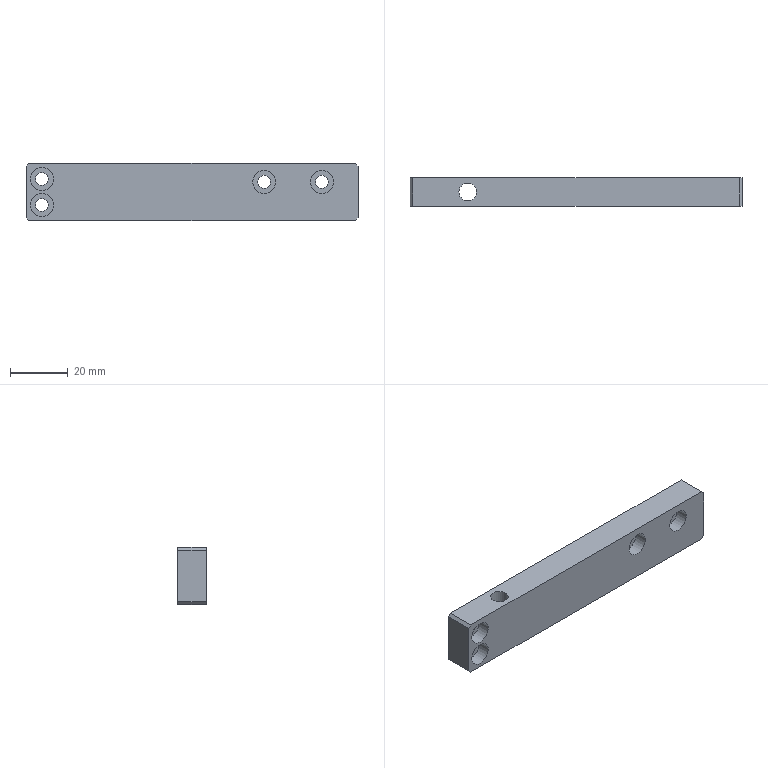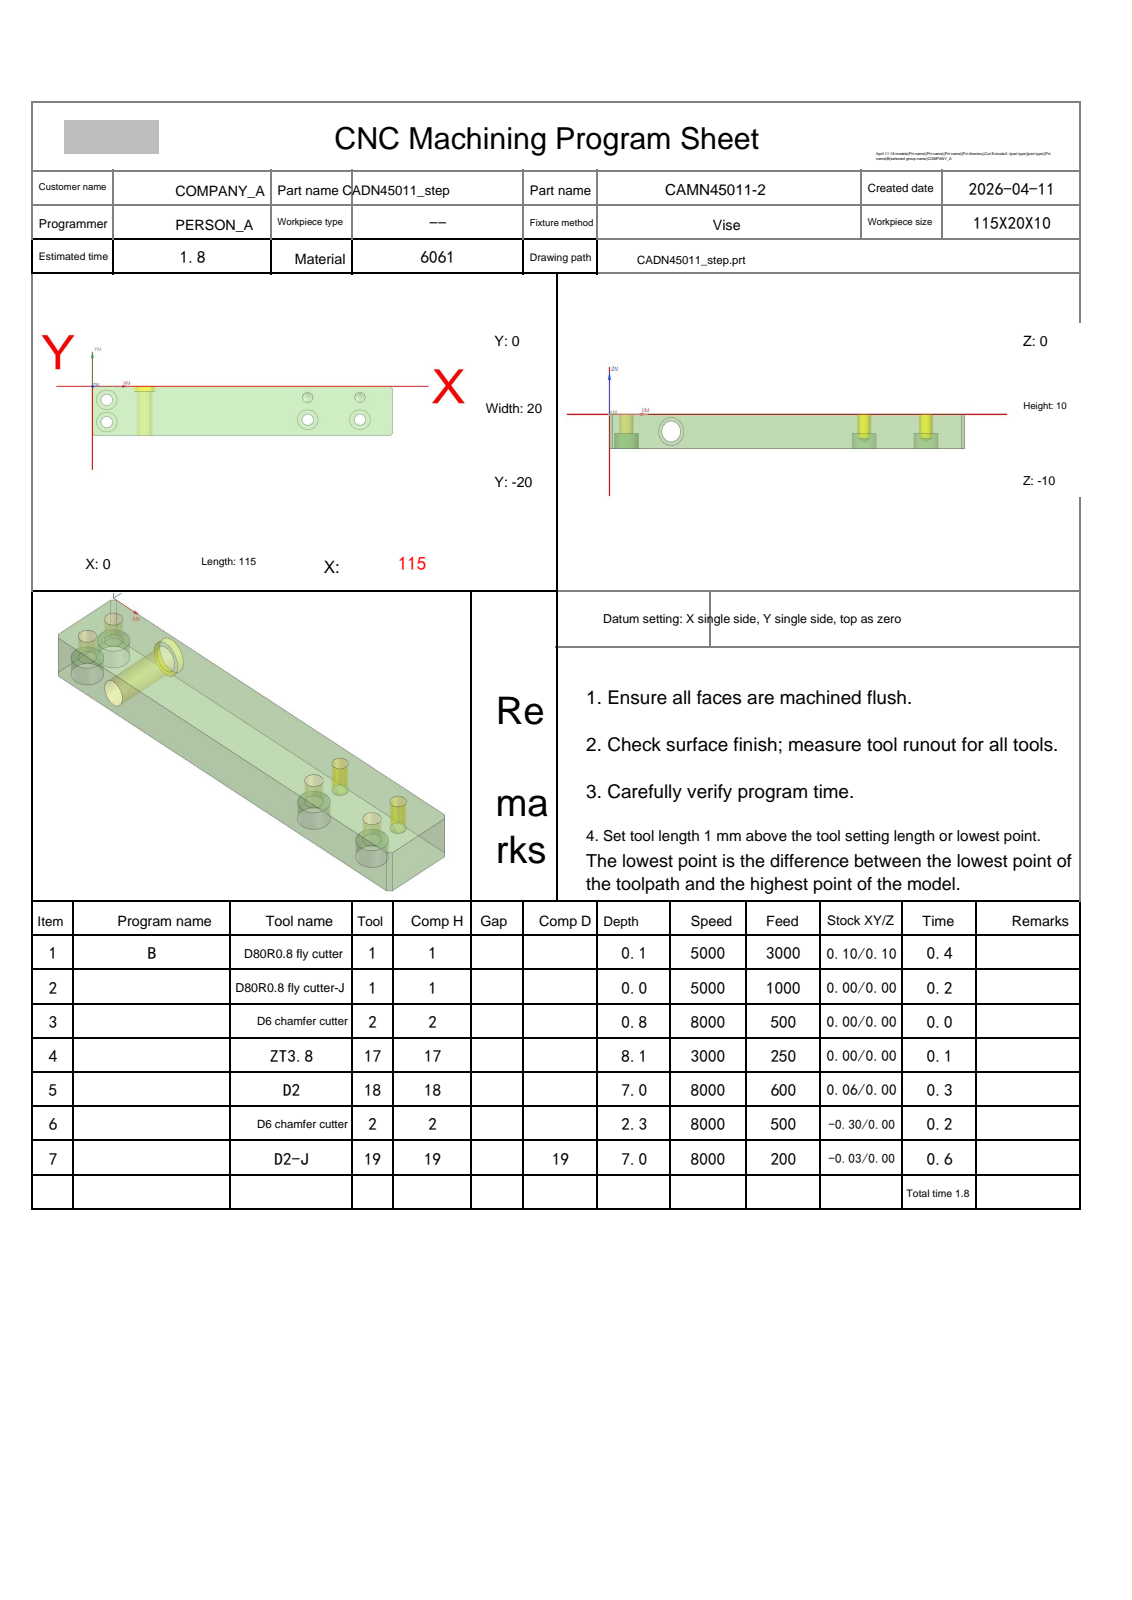NC program | NX | posted by the shop | part box 115 x 10 x 20 mm
Whole program:
%
O0001
(Machine time: 3.22 MIN)
(===Total Tool:5===)
(T1=D80R0.8 fly cutter D=80.  R=0.8  D-  H01 Z=0.    )
(T2=D6 chamfer cutter   D=6.   R=0.   D-  H02 Z=-2.3  )
(T17=ZT3.8  D=3.8  DR_a=118 D-  H17 Z=-8.1  )
(T18=D2     D=2.   R=0.   D-  H18 Z=-7.   )
(T19=D2-J   D=2.   R=0.   D19 H19 Z=-7.   )
G80 G90 G17 G49 G40
G91 G28 Z0
M01
N1 T01 M06
(D80R0.8 fly cutter  D=80. R=0.8 H=01 ce=0.10 di=0.10)
G00 G90 G54 X167.097 Y-10. M03 S5000
G43 H01 Z20.
M08
Z3.525
G01 Z1.525 F3000.
X155.097
X-40.097
X-52.097
Z3.525
G00 X167.097
Z3.05
G01 Z1.05
X155.097
X-40.097
X-52.097
Z3.05
G00 X167.097
Z2.575
G01 Z.575
X155.097
X-40.097
X-52.097
Z2.575
G00 X167.097
Z2.1
G01 Z.1
X155.097
X-40.097
X-52.097
Z2.1
G00 Z20.
G91 G28 Z0.0
M05
M09
G91 G28 Z0.0
M01
N2 T01 M06
(D80R0.8 fly cutter-J  D=80. R=0.8 H=01 ce=0.00 di=0.00)
G00 G90 G54 X166.999 Y-10. M03 S5000
G43 H01 Z20.
M08
Z2.
G01 Z0.0 F1000.
X154.999
X-39.999
X-51.999
Z2.
G00 Z20.
G91 G28 Z0.0
M05
M09
G91 G28 Z0.0
M01
N3 T02 M06
(D6 chamfer cutter  D=6. R=0. H=02 ce=0.00 di=0.00)
G00 G90 G54 X5.5 Y-5.5 M03 S8000
G43 H02 Z20.
M08
G98 G81 X5.5 Y-5.5 Z-.8 R1. F500.
Y-14.5
X82.5 Y-13.5
Y-4.5
X102.5
Y-13.5
G80
G00 Z20.
G91 G28 Z0.0
M05
M09
G91 G28 Z0.0
M01
N4 T17 M06
(ZT3.8 D=3.8 DR_a=118 H=17)
G00 G90 G54 X102.5 Y-4.5 M03 S3000
G43 H17 Z20.
M08
G98 G83 X102.5 Y-4.5 Z-8.102 R1. F250. Q2.
X82.5
G80
G00 Z20.
G91 G28 Z0.0
M05
M09
G91 G28 Z0.0
M01
N5 T18 M06
(D2  D=2. R=0. H=18 ce=0.06 di=0.00)
G00 G90 G54 X102.5 Y-4.5 M03 S8000
G43 H18 Z20.
M08
Z.5
G03 X102.97 Y-4.97 I.47 J0.0 F600.
X103.44 Y-4.5 I0.0 J.47
X103.44 Y-4.5 Z0.0 I-.94 J0.0
X103.44 Y-4.5 Z-.5 I-.94 J0.0
X103.44 Y-4.5 Z-1. I-.94 J0.0
X103.44 Y-4.5 Z-1.5 I-.94 J0.0
X103.44 Y-4.5 Z-2. I-.94 J0.0
X103.44 Y-4.5 Z-2.5 I-.94 J0.0
X103.44 Y-4.5 Z-3. I-.94 J0.0
X103.44 Y-4.5 Z-3.5 I-.94 J0.0
X103.44 Y-4.5 Z-4. I-.94 J0.0
X103.44 Y-4.5 Z-4.5 I-.94 J0.0
X103.44 Y-4.5 Z-5. I-.94 J0.0
X103.44 Y-4.5 Z-5.5 I-.94 J0.0
X103.44 Y-4.5 Z-6. I-.94 J0.0
X103.44 Y-4.5 Z-6.5 I-.94 J0.0
X103.44 Y-4.5 Z-7. I-.94 J0.0
X102.5 Y-3.56 I-.94 J0.0
X101.56 Y-4.5 I0.0 J-.94
X102.5 Y-5.44 I.94 J0.0
X103.44 Y-4.5 I0.0 J.94
X102.97 Y-4.03 I-.47 J0.0
X102.5 Y-4.5 I0.0 J-.47
G00 Z20.
X82.5
Z.5
G03 X82.97 Y-4.97 I.47 J0.0
X83.44 Y-4.5 I0.0 J.47
X83.44 Y-4.5 Z0.0 I-.94 J0.0
X83.44 Y-4.5 Z-.5 I-.94 J0.0
X83.44 Y-4.5 Z-1. I-.94 J0.0
X83.44 Y-4.5 Z-1.5 I-.94 J0.0
X83.44 Y-4.5 Z-2. I-.94 J0.0
X83.44 Y-4.5 Z-2.5 I-.94 J0.0
X83.44 Y-4.5 Z-3. I-.94 J0.0
X83.44 Y-4.5 Z-3.5 I-.94 J0.0
X83.44 Y-4.5 Z-4. I-.94 J0.0
X83.44 Y-4.5 Z-4.5 I-.94 J0.0
X83.44 Y-4.5 Z-5. I-.94 J0.0
X83.44 Y-4.5 Z-5.5 I-.94 J0.0
X83.44 Y-4.5 Z-6. I-.94 J0.0
X83.44 Y-4.5 Z-6.5 I-.94 J0.0
X83.44 Y-4.5 Z-7. I-.94 J0.0
X82.5 Y-3.56 I-.94 J0.0
X81.56 Y-4.5 I0.0 J-.94
X82.5 Y-5.44 I.94 J0.0
X83.44 Y-4.5 I0.0 J.94
X82.97 Y-4.03 I-.47 J0.0
X82.5 Y-4.5 I0.0 J-.47
G00 Z20.
G91 G28 Z0.0
M05
M09
G91 G28 Z0.0
M01
N6 T02 M06
(D6 chamfer cutter  D=6. R=0. H=02 ce=0.00 di=0.00)
G00 G90 G54 X102.5 Y-4.5 M03 S8000
G43 H02 Z20.
M08
G98 G81 X102.5 Y-4.5 Z-2.3 R3. F500.
X82.5
G80
G00 Z20.
G00 G90 X103.05 Y-13.482 M03 S8000
Z20.
Z-.5
G01 Z-1. F500.
X104. Y-13.45
G03 X102.5 Y-11.95 I-1.5 J0.0
X100.95 Y-13.5 I0.0 J-1.55
X102.5 Y-15.05 I1.55 J0.0
X104.05 Y-13.5 I0.0 J1.55
X102.5 Y-11.95 I-1.55 J0.0
X101. Y-13.45 I0.0 J-1.5
G01 X101.95 Y-13.482
Z-.5
G00 Z20.
X83.05
Z-.5
G01 Z-1.
X84. Y-13.45
G03 X82.5 Y-11.95 I-1.5 J0.0
X80.95 Y-13.5 I0.0 J-1.55
X82.5 Y-15.05 I1.55 J0.0
X84.05 Y-13.5 I0.0 J1.55
X82.5 Y-11.95 I-1.55 J0.0
X81. Y-13.45 I0.0 J-1.5
G01 X81.95 Y-13.482
Z-.5
G00 Z20.
X6.05 Y-14.482
Z-.5
G01 Z-1.
X7. Y-14.45
G03 X5.5 Y-12.95 I-1.5 J0.0
X3.95 Y-14.5 I0.0 J-1.55
X5.5 Y-16.05 I1.55 J0.0
X7.05 Y-14.5 I0.0 J1.55
X5.5 Y-12.95 I-1.55 J0.0
X4. Y-14.45 I0.0 J-1.5
G01 X4.95 Y-14.482
Z-.5
G00 Z20.
X6.05 Y-5.482
Z-.5
G01 Z-1.
X7. Y-5.45
G03 X5.5 Y-3.95 I-1.5 J0.0
X3.95 Y-5.5 I0.0 J-1.55
X5.5 Y-7.05 I1.55 J0.0
X7.05 Y-5.5 I0.0 J1.55
X5.5 Y-3.95 I-1.55 J0.0
X4. Y-5.45 I0.0 J-1.5
G01 X4.95 Y-5.482
Z-.5
G00 Z20.
G91 G28 Z0.0
M05
M09
G91 G28 Z0.0
M01
N7 T19 M06
(D2-J  D=2. R=0. H=19 ce=-0.03 di=0.00)
G00 G90 G54 X102.5 Y-4.5 M03 S8000
G43 H19 Z20.
M08
Z.5
G41 D19
G01 X102.575 Y-4.685 F200.
G03 X103.032 Y-4.993 I.457 J.185
X103.525 Y-4.5 I0.0 J.493
X103.525 Y-4.5 Z-.5 I-1.025 J0.0
X103.525 Y-4.5 Z-1.5 I-1.025 J0.0
X103.525 Y-4.5 Z-2.5 I-1.025 J0.0
X103.525 Y-4.5 Z-3.5 I-1.025 J0.0
X103.525 Y-4.5 Z-4.5 I-1.025 J0.0
X103.525 Y-4.5 Z-5.5 I-1.025 J0.0
X103.525 Y-4.5 Z-6.5 I-1.025 J0.0
X101.475 Y-4.5 Z-7. I-1.025 J0.0
X102.5 Y-5.525 I1.025 J0.0
X103.525 Y-4.5 I0.0 J1.025
X102.5 Y-3.475 I-1.025 J0.0
X101.475 Y-4.5 I0.0 J-1.025
X101.968 Y-4.993 I.493 J0.0
X102.425 Y-4.685 I0.0 J.493
G01 G40 X102.5 Y-4.5
G00 Z20.
X82.5
Z.5
G41 D19
G01 X82.575 Y-4.685
G03 X83.032 Y-4.993 I.457 J.185
X83.525 Y-4.5 I0.0 J.493
X83.525 Y-4.5 Z-.5 I-1.025 J0.0
X83.525 Y-4.5 Z-1.5 I-1.025 J0.0
X83.525 Y-4.5 Z-2.5 I-1.025 J0.0
X83.525 Y-4.5 Z-3.5 I-1.025 J0.0
X83.525 Y-4.5 Z-4.5 I-1.025 J0.0
X83.525 Y-4.5 Z-5.5 I-1.025 J0.0
X83.525 Y-4.5 Z-6.5 I-1.025 J0.0
X81.475 Y-4.5 Z-7. I-1.025 J0.0
X82.5 Y-5.525 I1.025 J0.0
X83.525 Y-4.5 I0.0 J1.025
X82.5 Y-3.475 I-1.025 J0.0
X81.475 Y-4.5 I0.0 J-1.025
X81.968 Y-4.993 I.493 J0.0
X82.425 Y-4.685 I0.0 J.493
G01 G40 X82.5 Y-4.5
G00 Z20.
M05
M09
G91 G28 Z0.0
G91 G28 Y0.0
M30
%